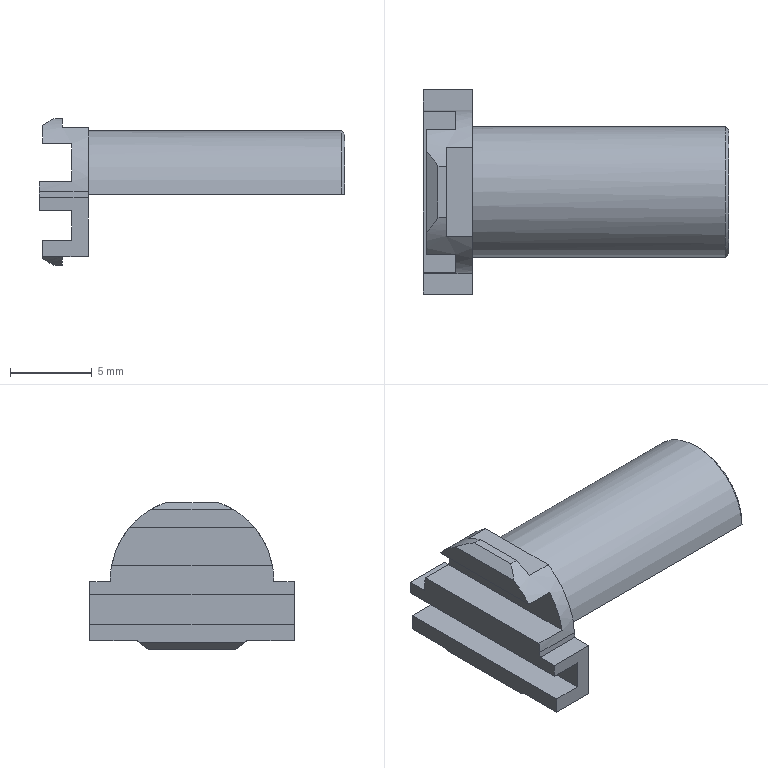Part | NX | features solid 2 | 1 solid | 65 faces | box 18.7 x 12.5 x 9 mm | volume 453.491 mm3 | plane 45 | cylinder 17 | spline 2 | cone 1 | commonest cylinder face diameters 0.3 x4 1.1 x4 10 x4 1.6 x1 1.9 x1 3.3 x1